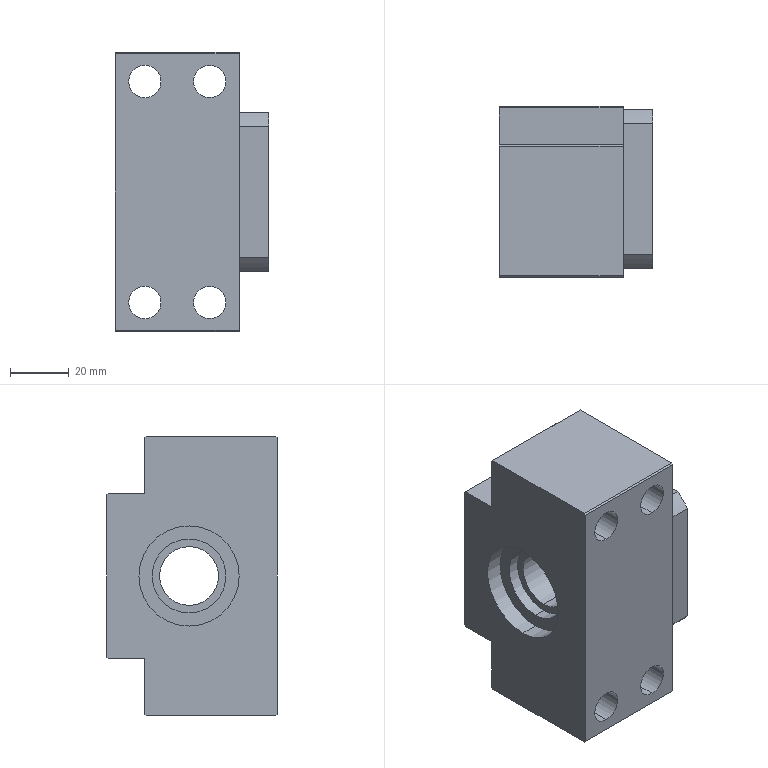Part | STEP file | 0244_Z_002_BSW20_1 | 1 solid | 114 faces | box 52 x 58 x 95 mm | volume 184374 mm3 | plane 66 | cylinder 48 | commonest cylinder face diameters 11 x16 10 x8 17 x8 25.1 x4 34 x4 70 x4